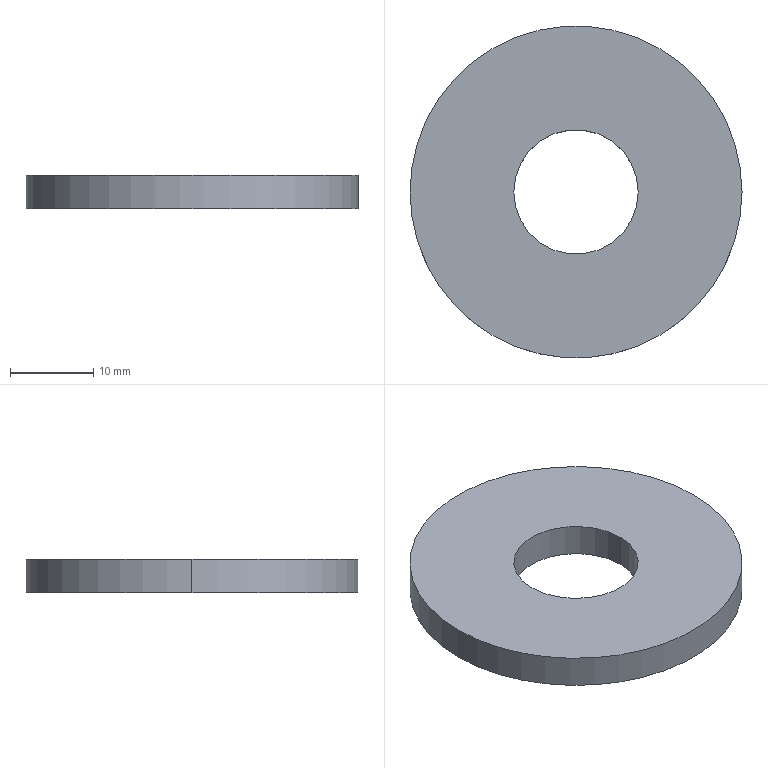Part | SolidWorks | features Extrusion 1 | 1 solid | 6 faces | box 40 x 40 x 4 mm | volume 4320 mm3 | cylinder 4 | plane 2 | commonest cylinder face diameters 15 x2 40 x2
STEP:
#1=CARTESIAN_POINT('',(-7.5,0.,4.));
#2=VERTEX_POINT('',#1);
#3=CARTESIAN_POINT('',(7.5,0.,4.));
#4=VERTEX_POINT('',#3);
#5=CARTESIAN_POINT('',(0.,0.,4.));
#6=DIRECTION('',(0.,0.,1.));
#7=DIRECTION('',(1.,0.,0.));
#8=AXIS2_PLACEMENT_3D('',#5,#6,#7);
#9=CIRCLE('',#8,7.5);
#10=EDGE_CURVE('',#2,#4,#9,.T.);
#11=ORIENTED_EDGE('',*,*,#10,.T.);
#12=CARTESIAN_POINT('',(7.5,0.,0.));
#13=VERTEX_POINT('',#12);
#14=CARTESIAN_POINT('',(7.5,0.,4.));
#15=DIRECTION('',(0.,0.,-1.));
#16=VECTOR('',#15,1000.);
#17=LINE('',#14,#16);
#18=EDGE_CURVE('',#4,#13,#17,.T.);
#19=ORIENTED_EDGE('',*,*,#18,.T.);
#20=CARTESIAN_POINT('',(-7.5,0.,0.));
#21=VERTEX_POINT('',#20);
#22=CARTESIAN_POINT('',(0.,0.,0.));
#23=DIRECTION('',(0.,0.,1.));
#24=DIRECTION('',(1.,0.,0.));
#25=AXIS2_PLACEMENT_3D('',#22,#23,#24);
#26=CIRCLE('',#25,7.5);
#27=EDGE_CURVE('',#21,#13,#26,.T.);
#28=ORIENTED_EDGE('',*,*,#27,.F.);
#29=CARTESIAN_POINT('',(-7.5,0.,4.));
#30=DIRECTION('',(0.,0.,-1.));
#31=VECTOR('',#30,1000.);
#32=LINE('',#29,#31);
#33=EDGE_CURVE('',#2,#21,#32,.T.);
#34=ORIENTED_EDGE('',*,*,#33,.F.);
#35=EDGE_LOOP('',(#11,#19,#28,#34));
#36=FACE_OUTER_BOUND('',#35,.T.);
#37=CARTESIAN_POINT('',(0.,0.,4.));
#38=DIRECTION('',(0.,0.,-1.));
#39=DIRECTION('',(-1.,0.,0.));
#40=AXIS2_PLACEMENT_3D('',#37,#38,#39);
#41=CYLINDRICAL_SURFACE('',#40,7.5);
#42=ADVANCED_FACE('',(#36),#41,.F.);
#43=CARTESIAN_POINT('',(20.,0.,4.));
#44=VERTEX_POINT('',#43);
#45=CARTESIAN_POINT('',(-20.,0.,4.));
#46=VERTEX_POINT('',#45);
#47=CARTESIAN_POINT('',(0.,0.,4.));
#48=DIRECTION('',(0.,0.,1.));
#49=DIRECTION('',(1.,0.,0.));
#50=AXIS2_PLACEMENT_3D('',#47,#48,#49);
#51=CIRCLE('',#50,20.);
#52=EDGE_CURVE('',#44,#46,#51,.T.);
#53=ORIENTED_EDGE('',*,*,#52,.F.);
#54=CARTESIAN_POINT('',(20.,0.,0.));
#55=VERTEX_POINT('',#54);
#56=CARTESIAN_POINT('',(20.,0.,4.));
#57=DIRECTION('',(0.,0.,-1.));
#58=VECTOR('',#57,1000.);
#59=LINE('',#56,#58);
#60=EDGE_CURVE('',#44,#55,#59,.T.);
#61=ORIENTED_EDGE('',*,*,#60,.T.);
#62=CARTESIAN_POINT('',(-20.,0.,0.));
#63=VERTEX_POINT('',#62);
#64=CARTESIAN_POINT('',(0.,0.,0.));
#65=DIRECTION('',(0.,0.,1.));
#66=DIRECTION('',(1.,0.,0.));
#67=AXIS2_PLACEMENT_3D('',#64,#65,#66);
#68=CIRCLE('',#67,20.);
#69=EDGE_CURVE('',#55,#63,#68,.T.);
#70=ORIENTED_EDGE('',*,*,#69,.T.);
#71=CARTESIAN_POINT('',(-20.,0.,4.));
#72=DIRECTION('',(0.,0.,-1.));
#73=VECTOR('',#72,1000.);
#74=LINE('',#71,#73);
#75=EDGE_CURVE('',#46,#63,#74,.T.);
#76=ORIENTED_EDGE('',*,*,#75,.F.);
#77=EDGE_LOOP('',(#53,#61,#70,#76));
#78=FACE_OUTER_BOUND('',#77,.T.);
#79=CARTESIAN_POINT('',(0.,0.,4.));
#80=DIRECTION('',(0.,0.,-1.));
#81=DIRECTION('',(-1.,0.,0.));
#82=AXIS2_PLACEMENT_3D('',#79,#80,#81);
#83=CYLINDRICAL_SURFACE('',#82,20.);
#84=ADVANCED_FACE('',(#78),#83,.T.);
#85=CARTESIAN_POINT('',(0.,0.,4.));
#86=DIRECTION('',(0.,0.,1.));
#87=DIRECTION('',(1.,0.,0.));
#88=AXIS2_PLACEMENT_3D('',#85,#86,#87);
#89=CIRCLE('',#88,20.);
#90=EDGE_CURVE('',#46,#44,#89,.T.);
#91=ORIENTED_EDGE('',*,*,#90,.T.);
#92=ORIENTED_EDGE('',*,*,#52,.T.);
#93=EDGE_LOOP('',(#91,#92));
#94=FACE_OUTER_BOUND('',#93,.T.);
#95=ORIENTED_EDGE('',*,*,#10,.F.);
#96=CARTESIAN_POINT('',(0.,0.,4.));
#97=DIRECTION('',(0.,0.,1.));
#98=DIRECTION('',(1.,0.,0.));
#99=AXIS2_PLACEMENT_3D('',#96,#97,#98);
#100=CIRCLE('',#99,7.5);
#101=EDGE_CURVE('',#4,#2,#100,.T.);
#102=ORIENTED_EDGE('',*,*,#101,.F.);
#103=EDGE_LOOP('',(#95,#102));
#104=FACE_BOUND('',#103,.T.);
#105=CARTESIAN_POINT('',(0.,0.,4.));
#106=DIRECTION('',(0.,0.,1.));
#107=DIRECTION('',(1.,0.,0.));
#108=AXIS2_PLACEMENT_3D('',#105,#106,#107);
#109=PLANE('',#108);
#110=ADVANCED_FACE('',(#94,#104),#109,.T.);
#111=CARTESIAN_POINT('',(0.,0.,0.));
#112=DIRECTION('',(0.,0.,1.));
#113=DIRECTION('',(1.,0.,0.));
#114=AXIS2_PLACEMENT_3D('',#111,#112,#113);
#115=CIRCLE('',#114,20.);
#116=EDGE_CURVE('',#63,#55,#115,.T.);
#117=ORIENTED_EDGE('',*,*,#116,.F.);
#118=ORIENTED_EDGE('',*,*,#69,.F.);
#119=EDGE_LOOP('',(#117,#118));
#120=FACE_OUTER_BOUND('',#119,.T.);
#121=ORIENTED_EDGE('',*,*,#27,.T.);
#122=CARTESIAN_POINT('',(0.,0.,0.));
#123=DIRECTION('',(0.,0.,1.));
#124=DIRECTION('',(1.,0.,0.));
#125=AXIS2_PLACEMENT_3D('',#122,#123,#124);
#126=CIRCLE('',#125,7.5);
#127=EDGE_CURVE('',#13,#21,#126,.T.);
#128=ORIENTED_EDGE('',*,*,#127,.T.);
#129=EDGE_LOOP('',(#121,#128));
#130=FACE_BOUND('',#129,.T.);
#131=CARTESIAN_POINT('',(0.,0.,0.));
#132=DIRECTION('',(0.,0.,1.));
#133=DIRECTION('',(1.,0.,0.));
#134=AXIS2_PLACEMENT_3D('',#131,#132,#133);
#135=PLANE('',#134);
#136=ADVANCED_FACE('',(#120,#130),#135,.F.);
#137=ORIENTED_EDGE('',*,*,#60,.F.);
#138=ORIENTED_EDGE('',*,*,#90,.F.);
#139=ORIENTED_EDGE('',*,*,#75,.T.);
#140=ORIENTED_EDGE('',*,*,#116,.T.);
#141=EDGE_LOOP('',(#137,#138,#139,#140));
#142=FACE_OUTER_BOUND('',#141,.T.);
#143=CARTESIAN_POINT('',(0.,0.,4.));
#144=DIRECTION('',(0.,0.,-1.));
#145=DIRECTION('',(-1.,0.,0.));
#146=AXIS2_PLACEMENT_3D('',#143,#144,#145);
#147=CYLINDRICAL_SURFACE('',#146,20.);
#148=ADVANCED_FACE('',(#142),#147,.T.);
#149=ORIENTED_EDGE('',*,*,#18,.F.);
#150=ORIENTED_EDGE('',*,*,#101,.T.);
#151=ORIENTED_EDGE('',*,*,#33,.T.);
#152=ORIENTED_EDGE('',*,*,#127,.F.);
#153=EDGE_LOOP('',(#149,#150,#151,#152));
#154=FACE_OUTER_BOUND('',#153,.T.);
#155=CARTESIAN_POINT('',(0.,0.,4.));
#156=DIRECTION('',(0.,0.,-1.));
#157=DIRECTION('',(-1.,0.,0.));
#158=AXIS2_PLACEMENT_3D('',#155,#156,#157);
#159=CYLINDRICAL_SURFACE('',#158,7.5);
#160=ADVANCED_FACE('',(#154),#159,.F.);
#161=CLOSED_SHELL('',(#42,#84,#110,#136,#148,#160));
#162=MANIFOLD_SOLID_BREP('',#161);
#163=CARTESIAN_POINT('',(0.,0.,0.));
#164=DIRECTION('',(0.,0.,1.));
#165=DIRECTION('',(1.,0.,0.));
#166=AXIS2_PLACEMENT_3D('',#163,#164,#165);
#167=(LENGTH_UNIT()NAMED_UNIT(*)SI_UNIT(.MILLI.,.METRE.));
#168=UNCERTAINTY_MEASURE_WITH_UNIT(LENGTH_MEASURE(0.00001),#167,'','');
#169=(NAMED_UNIT(*)PLANE_ANGLE_UNIT()SI_UNIT($,.RADIAN.));
#170=(NAMED_UNIT(*)SI_UNIT($,.STERADIAN.)SOLID_ANGLE_UNIT());
#171=(GEOMETRIC_REPRESENTATION_CONTEXT(3)GLOBAL_UNCERTAINTY_ASSIGNED_CONTEXT((#168))GLOBAL_UNIT_ASSIGNED_CONTEXT((#167,#169,#170))REPRESENTATION_CONTEXT('',''));
#172=ADVANCED_BREP_SHAPE_REPRESENTATION('',(#162,#166),#171);